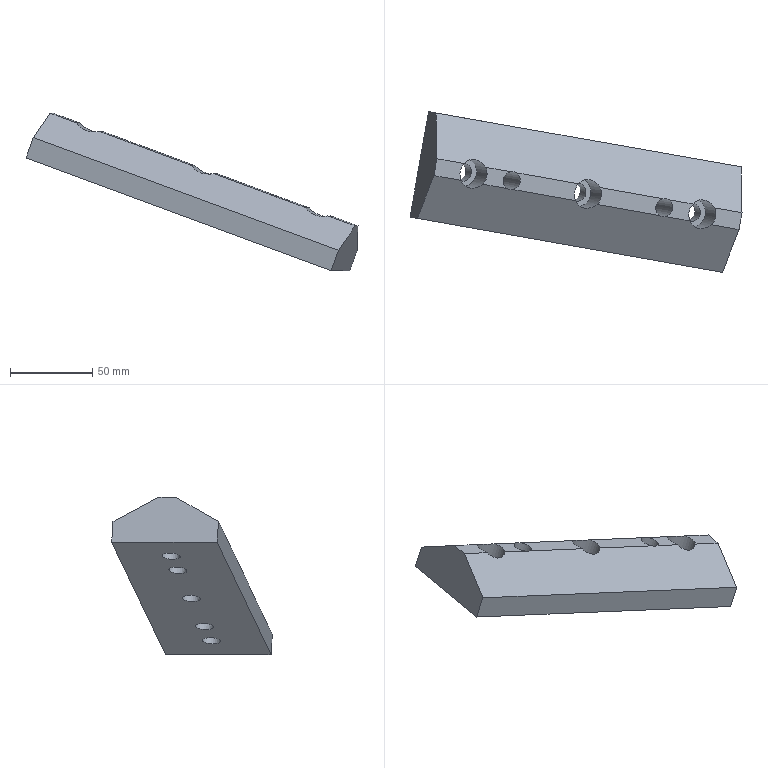Part | NX | features solid 2 | 1 solid | 24 faces | box 201.397 x 97.434 x 95.655 mm | volume 269020 mm3 | plane 16 | cylinder 8 | commonest cylinder face diameters 11 x5 17.5 x3
STEP:
#1=CARTESIAN_POINT('',(-972.407,367.24,-198.041));
#2=VERTEX_POINT('',#1);
#3=CARTESIAN_POINT('',(-1010.495,373.956,-183.964));
#4=VERTEX_POINT('',#3);
#5=CARTESIAN_POINT('',(-873.35,349.774,-234.651));
#6=DIRECTION('',(-0.9254,0.1632,0.342));
#7=VECTOR('',#6,1000.);
#8=LINE('',#5,#7);
#9=EDGE_CURVE('',#2,#4,#8,.T.);
#10=ORIENTED_EDGE('',*,*,#9,.T.);
#11=CARTESIAN_POINT('',(-1012.299,363.722,-183.964));
#12=VERTEX_POINT('',#11);
#13=CARTESIAN_POINT('',(-1013.065,369.133,-183.348));
#14=DIRECTION('',(-0.3368,0.05939,-0.9397));
#15=DIRECTION('',(-0.9254,0.1632,0.342));
#16=AXIS2_PLACEMENT_3D('',#13,#14,#15);
#17=CIRCLE('',#16,5.5);
#18=EDGE_CURVE('',#4,#12,#17,.T.);
#19=ORIENTED_EDGE('',*,*,#18,.T.);
#20=CARTESIAN_POINT('',(-974.212,357.006,-198.041));
#21=VERTEX_POINT('',#20);
#22=CARTESIAN_POINT('',(-875.155,339.54,-234.651));
#23=DIRECTION('',(-0.9254,0.1632,0.342));
#24=VECTOR('',#23,1000.);
#25=LINE('',#22,#24);
#26=EDGE_CURVE('',#21,#12,#25,.T.);
#27=ORIENTED_EDGE('',*,*,#26,.F.);
#28=CARTESIAN_POINT('',(-966.794,360.974,-200.449));
#29=DIRECTION('',(0.3368,-0.05939,0.9397));
#30=DIRECTION('',(0.9254,-0.1632,-0.342));
#31=AXIS2_PLACEMENT_3D('',#28,#29,#30);
#32=CIRCLE('',#31,8.75);
#33=EDGE_CURVE('',#2,#21,#32,.T.);
#34=ORIENTED_EDGE('',*,*,#33,.F.);
#35=EDGE_LOOP('',(#10,#19,#27,#34));
#36=FACE_BOUND('',#35,.T.);
#37=CARTESIAN_POINT('',(-875.155,339.54,-234.651));
#38=DIRECTION('',(0.3368,-0.05939,0.9397));
#39=DIRECTION('',(0.9254,-0.1632,-0.342));
#40=AXIS2_PLACEMENT_3D('',#37,#38,#39);
#41=PLANE('',#40);
#42=ADVANCED_FACE('',(#36),#41,.T.);
#43=CARTESIAN_POINT('',(-1051.058,375.832,-200.167));
#44=VERTEX_POINT('',#43);
#45=CARTESIAN_POINT('',(-1045.969,374.935,-202.048));
#46=DIRECTION('',(0.3368,-0.05939,0.9397));
#47=DIRECTION('',(-0.9254,0.1632,0.342));
#48=AXIS2_PLACEMENT_3D('',#45,#46,#47);
#49=CIRCLE('',#48,5.5);
#50=EDGE_CURVE('',#44,#44,#49,.T.);
#51=ORIENTED_EDGE('',*,*,#50,.T.);
#52=EDGE_LOOP('',(#51));
#53=FACE_BOUND('',#52,.T.);
#54=CARTESIAN_POINT('',(-1027.923,371.753,-208.718));
#55=VERTEX_POINT('',#54);
#56=CARTESIAN_POINT('',(-1022.833,370.855,-210.599));
#57=DIRECTION('',(-0.3368,0.05939,-0.9397));
#58=DIRECTION('',(-0.9254,0.1632,0.342));
#59=AXIS2_PLACEMENT_3D('',#56,#57,#58);
#60=CIRCLE('',#59,5.5);
#61=EDGE_CURVE('',#55,#55,#60,.T.);
#62=ORIENTED_EDGE('',*,*,#61,.F.);
#63=EDGE_LOOP('',(#62));
#64=FACE_BOUND('',#63,.T.);
#65=CARTESIAN_POINT('',(-981.652,363.594,-225.819));
#66=VERTEX_POINT('',#65);
#67=CARTESIAN_POINT('',(-976.562,362.697,-227.7));
#68=DIRECTION('',(0.3368,-0.05939,0.9397));
#69=DIRECTION('',(-0.9254,0.1632,0.342));
#70=AXIS2_PLACEMENT_3D('',#67,#68,#69);
#71=CIRCLE('',#70,5.5);
#72=EDGE_CURVE('',#66,#66,#71,.T.);
#73=ORIENTED_EDGE('',*,*,#72,.T.);
#74=EDGE_LOOP('',(#73));
#75=FACE_BOUND('',#74,.T.);
#76=CARTESIAN_POINT('',(-889.664,314.373,-261.902));
#77=VERTEX_POINT('',#76);
#78=CARTESIAN_POINT('',(-1074.747,347.008,-193.498));
#79=VERTEX_POINT('',#78);
#80=CARTESIAN_POINT('',(-889.664,314.373,-261.902));
#81=DIRECTION('',(-0.9254,0.1632,0.342));
#82=VECTOR('',#81,1000.);
#83=LINE('',#80,#82);
#84=EDGE_CURVE('',#77,#79,#83,.T.);
#85=ORIENTED_EDGE('',*,*,#84,.T.);
#86=CARTESIAN_POINT('',(-1063.46,411.021,-193.498));
#87=VERTEX_POINT('',#86);
#88=CARTESIAN_POINT('',(-1074.747,347.008,-193.498));
#89=DIRECTION('',(0.1736,0.9848,0.));
#90=VECTOR('',#89,1000.);
#91=LINE('',#88,#90);
#92=EDGE_CURVE('',#79,#87,#91,.T.);
#93=ORIENTED_EDGE('',*,*,#92,.T.);
#94=CARTESIAN_POINT('',(-878.377,378.385,-261.902));
#95=VERTEX_POINT('',#94);
#96=CARTESIAN_POINT('',(-878.377,378.385,-261.902));
#97=DIRECTION('',(-0.9254,0.1632,0.342));
#98=VECTOR('',#97,1000.);
#99=LINE('',#96,#98);
#100=EDGE_CURVE('',#95,#87,#99,.T.);
#101=ORIENTED_EDGE('',*,*,#100,.F.);
#102=CARTESIAN_POINT('',(-889.664,314.373,-261.902));
#103=DIRECTION('',(0.1736,0.9848,0.));
#104=VECTOR('',#103,1000.);
#105=LINE('',#102,#104);
#106=EDGE_CURVE('',#77,#95,#105,.T.);
#107=ORIENTED_EDGE('',*,*,#106,.F.);
#108=EDGE_LOOP('',(#85,#93,#101,#107));
#109=FACE_BOUND('',#108,.T.);
#110=CARTESIAN_POINT('',(-935.381,355.435,-242.92));
#111=VERTEX_POINT('',#110);
#112=CARTESIAN_POINT('',(-930.291,354.538,-244.801));
#113=DIRECTION('',(-0.3368,0.05939,-0.9397));
#114=DIRECTION('',(-0.9254,0.1632,0.342));
#115=AXIS2_PLACEMENT_3D('',#112,#113,#114);
#116=CIRCLE('',#115,5.5);
#117=EDGE_CURVE('',#111,#111,#116,.T.);
#118=ORIENTED_EDGE('',*,*,#117,.F.);
#119=EDGE_LOOP('',(#118));
#120=FACE_BOUND('',#119,.T.);
#121=CARTESIAN_POINT('',(-912.246,351.356,-251.47));
#122=VERTEX_POINT('',#121);
#123=CARTESIAN_POINT('',(-907.156,350.459,-253.351));
#124=DIRECTION('',(0.3368,-0.05939,0.9397));
#125=DIRECTION('',(-0.9254,0.1632,0.342));
#126=AXIS2_PLACEMENT_3D('',#123,#124,#125);
#127=CIRCLE('',#126,5.5);
#128=EDGE_CURVE('',#122,#122,#127,.T.);
#129=ORIENTED_EDGE('',*,*,#128,.T.);
#130=EDGE_LOOP('',(#129));
#131=FACE_BOUND('',#130,.T.);
#132=CARTESIAN_POINT('',(-889.664,314.373,-261.902));
#133=DIRECTION('',(0.3368,-0.05939,0.9397));
#134=DIRECTION('',(-0.1736,-0.9848,0.));
#135=AXIS2_PLACEMENT_3D('',#132,#133,#134);
#136=PLANE('',#135);
#137=ADVANCED_FACE('',(#53,#64,#75,#109,#120,#131),#136,.F.);
#138=CARTESIAN_POINT('',(-1013.831,374.545,-182.731));
#139=VERTEX_POINT('',#138);
#140=CARTESIAN_POINT('',(-1012.055,368.955,-180.529));
#141=DIRECTION('',(0.3785,0.441,0.8138));
#142=DIRECTION('',(-0.01803,0.8826,-0.4698));
#143=AXIS2_PLACEMENT_3D('',#140,#141,#142);
#144=ELLIPSE('',#143,6.351,5.5);
#145=EDGE_CURVE('',#4,#139,#144,.T.);
#146=ORIENTED_EDGE('',*,*,#145,.F.);
#147=ORIENTED_EDGE('',*,*,#9,.F.);
#148=CARTESIAN_POINT('',(-959.377,364.943,-202.857));
#149=VERTEX_POINT('',#148);
#150=CARTESIAN_POINT('',(-965.784,360.796,-197.63));
#151=DIRECTION('',(0.3785,0.441,0.8138));
#152=DIRECTION('',(-0.01803,0.8826,-0.4698));
#153=AXIS2_PLACEMENT_3D('',#150,#151,#152);
#154=ELLIPSE('',#153,10.104,8.75);
#155=EDGE_CURVE('',#149,#2,#154,.T.);
#156=ORIENTED_EDGE('',*,*,#155,.F.);
#157=CARTESIAN_POINT('',(-921.29,358.227,-216.933));
#158=VERTEX_POINT('',#157);
#159=CARTESIAN_POINT('',(-873.35,349.774,-234.651));
#160=DIRECTION('',(-0.9254,0.1632,0.342));
#161=VECTOR('',#160,1000.);
#162=LINE('',#159,#161);
#163=EDGE_CURVE('',#158,#149,#162,.T.);
#164=ORIENTED_EDGE('',*,*,#163,.F.);
#165=CARTESIAN_POINT('',(-917.953,357.639,-218.166));
#166=VERTEX_POINT('',#165);
#167=CARTESIAN_POINT('',(-919.513,352.637,-214.731));
#168=DIRECTION('',(0.3785,0.441,0.8138));
#169=DIRECTION('',(-0.01803,0.8826,-0.4698));
#170=AXIS2_PLACEMENT_3D('',#167,#168,#169);
#171=ELLIPSE('',#170,6.351,5.5);
#172=EDGE_CURVE('',#166,#158,#171,.T.);
#173=ORIENTED_EDGE('',*,*,#172,.F.);
#174=CARTESIAN_POINT('',(-903.001,355.002,-223.692));
#175=VERTEX_POINT('',#174);
#176=CARTESIAN_POINT('',(-873.35,349.774,-234.651));
#177=DIRECTION('',(-0.9254,0.1632,0.342));
#178=VECTOR('',#177,1000.);
#179=LINE('',#176,#178);
#180=EDGE_CURVE('',#175,#166,#179,.T.);
#181=ORIENTED_EDGE('',*,*,#180,.F.);
#182=CARTESIAN_POINT('',(-889.971,352.705,-228.508));
#183=VERTEX_POINT('',#182);
#184=CARTESIAN_POINT('',(-896.378,348.558,-223.281));
#185=DIRECTION('',(0.3785,0.441,0.8138));
#186=DIRECTION('',(-0.01803,0.8826,-0.4698));
#187=AXIS2_PLACEMENT_3D('',#184,#185,#186);
#188=ELLIPSE('',#187,10.104,8.75);
#189=EDGE_CURVE('',#183,#175,#188,.T.);
#190=ORIENTED_EDGE('',*,*,#189,.F.);
#191=CARTESIAN_POINT('',(-873.35,349.774,-234.651));
#192=VERTEX_POINT('',#191);
#193=CARTESIAN_POINT('',(-873.35,349.774,-234.651));
#194=DIRECTION('',(-0.9254,0.1632,0.342));
#195=VECTOR('',#194,1000.);
#196=LINE('',#193,#195);
#197=EDGE_CURVE('',#192,#183,#196,.T.);
#198=ORIENTED_EDGE('',*,*,#197,.F.);
#199=CARTESIAN_POINT('',(-873.919,377.599,-249.464));
#200=VERTEX_POINT('',#199);
#201=CARTESIAN_POINT('',(-873.35,349.774,-234.651));
#202=DIRECTION('',(-0.01803,0.8826,-0.4698));
#203=VECTOR('',#202,1000.);
#204=LINE('',#201,#203);
#205=EDGE_CURVE('',#192,#200,#204,.T.);
#206=ORIENTED_EDGE('',*,*,#205,.T.);
#207=CARTESIAN_POINT('',(-1059.002,410.234,-181.06));
#208=VERTEX_POINT('',#207);
#209=CARTESIAN_POINT('',(-873.919,377.599,-249.464));
#210=DIRECTION('',(-0.9254,0.1632,0.342));
#211=VECTOR('',#210,1000.);
#212=LINE('',#209,#211);
#213=EDGE_CURVE('',#200,#208,#212,.T.);
#214=ORIENTED_EDGE('',*,*,#213,.T.);
#215=CARTESIAN_POINT('',(-1058.434,382.409,-166.247));
#216=VERTEX_POINT('',#215);
#217=CARTESIAN_POINT('',(-1058.434,382.409,-166.247));
#218=DIRECTION('',(-0.01803,0.8826,-0.4698));
#219=VECTOR('',#218,1000.);
#220=LINE('',#217,#219);
#221=EDGE_CURVE('',#216,#208,#220,.T.);
#222=ORIENTED_EDGE('',*,*,#221,.F.);
#223=CARTESIAN_POINT('',(-1041.813,379.479,-172.389));
#224=VERTEX_POINT('',#223);
#225=CARTESIAN_POINT('',(-873.35,349.774,-234.651));
#226=DIRECTION('',(-0.9254,0.1632,0.342));
#227=VECTOR('',#226,1000.);
#228=LINE('',#225,#227);
#229=EDGE_CURVE('',#224,#216,#228,.T.);
#230=ORIENTED_EDGE('',*,*,#229,.F.);
#231=CARTESIAN_POINT('',(-1028.783,377.181,-177.205));
#232=VERTEX_POINT('',#231);
#233=CARTESIAN_POINT('',(-1035.19,373.034,-171.978));
#234=DIRECTION('',(0.3785,0.441,0.8138));
#235=DIRECTION('',(-0.01803,0.8826,-0.4698));
#236=AXIS2_PLACEMENT_3D('',#233,#234,#235);
#237=ELLIPSE('',#236,10.104,8.75);
#238=EDGE_CURVE('',#232,#224,#237,.T.);
#239=ORIENTED_EDGE('',*,*,#238,.F.);
#240=CARTESIAN_POINT('',(-873.35,349.774,-234.651));
#241=DIRECTION('',(-0.9254,0.1632,0.342));
#242=VECTOR('',#241,1000.);
#243=LINE('',#240,#242);
#244=EDGE_CURVE('',#139,#232,#243,.T.);
#245=ORIENTED_EDGE('',*,*,#244,.F.);
#246=EDGE_LOOP('',(#146,#147,#156,#164,#173,#181,#190,#198,#206,#214,#222,#230,#239,#245));
#247=FACE_BOUND('',#246,.T.);
#248=CARTESIAN_POINT('',(-873.35,349.774,-234.651));
#249=DIRECTION('',(0.3785,0.441,0.8138));
#250=DIRECTION('',(0.01803,-0.8826,0.4698));
#251=AXIS2_PLACEMENT_3D('',#248,#249,#250);
#252=PLANE('',#251);
#253=ADVANCED_FACE('',(#247),#252,.T.);
#254=ORIENTED_EDGE('',*,*,#26,.T.);
#255=CARTESIAN_POINT('',(-1015.636,364.31,-182.731));
#256=VERTEX_POINT('',#255);
#257=CARTESIAN_POINT('',(-1012.055,368.955,-180.529));
#258=DIRECTION('',(-0.2049,0.5438,-0.8138));
#259=DIRECTION('',(-0.3188,-0.8232,-0.4698));
#260=AXIS2_PLACEMENT_3D('',#257,#258,#259);
#261=ELLIPSE('',#260,6.351,5.5);
#262=EDGE_CURVE('',#12,#256,#261,.T.);
#263=ORIENTED_EDGE('',*,*,#262,.T.);
#264=CARTESIAN_POINT('',(-1030.588,366.947,-177.205));
#265=VERTEX_POINT('',#264);
#266=CARTESIAN_POINT('',(-875.155,339.54,-234.651));
#267=DIRECTION('',(-0.9254,0.1632,0.342));
#268=VECTOR('',#267,1000.);
#269=LINE('',#266,#268);
#270=EDGE_CURVE('',#256,#265,#269,.T.);
#271=ORIENTED_EDGE('',*,*,#270,.T.);
#272=CARTESIAN_POINT('',(-1043.618,369.244,-172.389));
#273=VERTEX_POINT('',#272);
#274=CARTESIAN_POINT('',(-1035.19,373.034,-171.978));
#275=DIRECTION('',(-0.2049,0.5438,-0.8138));
#276=DIRECTION('',(-0.3188,-0.8232,-0.4698));
#277=AXIS2_PLACEMENT_3D('',#274,#275,#276);
#278=ELLIPSE('',#277,10.104,8.75);
#279=EDGE_CURVE('',#265,#273,#278,.T.);
#280=ORIENTED_EDGE('',*,*,#279,.T.);
#281=CARTESIAN_POINT('',(-1060.238,372.175,-166.247));
#282=VERTEX_POINT('',#281);
#283=CARTESIAN_POINT('',(-875.155,339.54,-234.651));
#284=DIRECTION('',(-0.9254,0.1632,0.342));
#285=VECTOR('',#284,1000.);
#286=LINE('',#283,#285);
#287=EDGE_CURVE('',#273,#282,#286,.T.);
#288=ORIENTED_EDGE('',*,*,#287,.T.);
#289=CARTESIAN_POINT('',(-1070.289,346.222,-181.06));
#290=VERTEX_POINT('',#289);
#291=CARTESIAN_POINT('',(-1060.238,372.175,-166.247));
#292=DIRECTION('',(-0.3188,-0.8232,-0.4698));
#293=VECTOR('',#292,1000.);
#294=LINE('',#291,#293);
#295=EDGE_CURVE('',#282,#290,#294,.T.);
#296=ORIENTED_EDGE('',*,*,#295,.T.);
#297=CARTESIAN_POINT('',(-885.206,313.587,-249.464));
#298=VERTEX_POINT('',#297);
#299=CARTESIAN_POINT('',(-885.206,313.587,-249.464));
#300=DIRECTION('',(-0.9254,0.1632,0.342));
#301=VECTOR('',#300,1000.);
#302=LINE('',#299,#301);
#303=EDGE_CURVE('',#298,#290,#302,.T.);
#304=ORIENTED_EDGE('',*,*,#303,.F.);
#305=CARTESIAN_POINT('',(-875.155,339.54,-234.651));
#306=VERTEX_POINT('',#305);
#307=CARTESIAN_POINT('',(-875.155,339.54,-234.651));
#308=DIRECTION('',(-0.3188,-0.8232,-0.4698));
#309=VECTOR('',#308,1000.);
#310=LINE('',#307,#309);
#311=EDGE_CURVE('',#306,#298,#310,.T.);
#312=ORIENTED_EDGE('',*,*,#311,.F.);
#313=CARTESIAN_POINT('',(-891.775,342.47,-228.508));
#314=VERTEX_POINT('',#313);
#315=CARTESIAN_POINT('',(-875.155,339.54,-234.651));
#316=DIRECTION('',(-0.9254,0.1632,0.342));
#317=VECTOR('',#316,1000.);
#318=LINE('',#315,#317);
#319=EDGE_CURVE('',#306,#314,#318,.T.);
#320=ORIENTED_EDGE('',*,*,#319,.T.);
#321=CARTESIAN_POINT('',(-904.805,344.768,-223.692));
#322=VERTEX_POINT('',#321);
#323=CARTESIAN_POINT('',(-896.378,348.558,-223.281));
#324=DIRECTION('',(-0.2049,0.5438,-0.8138));
#325=DIRECTION('',(-0.3188,-0.8232,-0.4698));
#326=AXIS2_PLACEMENT_3D('',#323,#324,#325);
#327=ELLIPSE('',#326,10.104,8.75);
#328=EDGE_CURVE('',#314,#322,#327,.T.);
#329=ORIENTED_EDGE('',*,*,#328,.T.);
#330=CARTESIAN_POINT('',(-919.758,347.404,-218.166));
#331=VERTEX_POINT('',#330);
#332=CARTESIAN_POINT('',(-875.155,339.54,-234.651));
#333=DIRECTION('',(-0.9254,0.1632,0.342));
#334=VECTOR('',#333,1000.);
#335=LINE('',#332,#334);
#336=EDGE_CURVE('',#322,#331,#335,.T.);
#337=ORIENTED_EDGE('',*,*,#336,.T.);
#338=CARTESIAN_POINT('',(-923.094,347.993,-216.933));
#339=VERTEX_POINT('',#338);
#340=CARTESIAN_POINT('',(-919.513,352.637,-214.731));
#341=DIRECTION('',(-0.2049,0.5438,-0.8138));
#342=DIRECTION('',(-0.3188,-0.8232,-0.4698));
#343=AXIS2_PLACEMENT_3D('',#340,#341,#342);
#344=ELLIPSE('',#343,6.351,5.5);
#345=EDGE_CURVE('',#331,#339,#344,.T.);
#346=ORIENTED_EDGE('',*,*,#345,.T.);
#347=CARTESIAN_POINT('',(-961.182,354.708,-202.857));
#348=VERTEX_POINT('',#347);
#349=CARTESIAN_POINT('',(-875.155,339.54,-234.651));
#350=DIRECTION('',(-0.9254,0.1632,0.342));
#351=VECTOR('',#350,1000.);
#352=LINE('',#349,#351);
#353=EDGE_CURVE('',#339,#348,#352,.T.);
#354=ORIENTED_EDGE('',*,*,#353,.T.);
#355=CARTESIAN_POINT('',(-965.784,360.796,-197.63));
#356=DIRECTION('',(-0.2049,0.5438,-0.8138));
#357=DIRECTION('',(-0.3188,-0.8232,-0.4698));
#358=AXIS2_PLACEMENT_3D('',#355,#356,#357);
#359=ELLIPSE('',#358,10.104,8.75);
#360=EDGE_CURVE('',#348,#21,#359,.T.);
#361=ORIENTED_EDGE('',*,*,#360,.T.);
#362=EDGE_LOOP('',(#254,#263,#271,#280,#288,#296,#304,#312,#320,#329,#337,#346,#354,#361));
#363=FACE_BOUND('',#362,.T.);
#364=CARTESIAN_POINT('',(-875.155,339.54,-234.651));
#365=DIRECTION('',(0.2049,-0.5438,0.8138));
#366=DIRECTION('',(0.3188,0.8232,0.4698));
#367=AXIS2_PLACEMENT_3D('',#364,#365,#366);
#368=PLANE('',#367);
#369=ADVANCED_FACE('',(#363),#368,.T.);
#370=CARTESIAN_POINT('',(-966.794,360.974,-200.449));
#371=DIRECTION('',(-0.3368,0.05939,-0.9397));
#372=DIRECTION('',(-0.9254,0.1632,0.342));
#373=AXIS2_PLACEMENT_3D('',#370,#371,#372);
#374=CIRCLE('',#373,8.75);
#375=EDGE_CURVE('',#149,#348,#374,.T.);
#376=ORIENTED_EDGE('',*,*,#375,.T.);
#377=ORIENTED_EDGE('',*,*,#353,.F.);
#378=CARTESIAN_POINT('',(-920.524,352.816,-217.55));
#379=DIRECTION('',(-0.3368,0.05939,-0.9397));
#380=DIRECTION('',(-0.9254,0.1632,0.342));
#381=AXIS2_PLACEMENT_3D('',#378,#379,#380);
#382=CIRCLE('',#381,5.5);
#383=EDGE_CURVE('',#339,#158,#382,.T.);
#384=ORIENTED_EDGE('',*,*,#383,.T.);
#385=ORIENTED_EDGE('',*,*,#163,.T.);
#386=EDGE_LOOP('',(#376,#377,#384,#385));
#387=FACE_BOUND('',#386,.T.);
#388=CARTESIAN_POINT('',(-875.155,339.54,-234.651));
#389=DIRECTION('',(0.3368,-0.05939,0.9397));
#390=DIRECTION('',(0.9254,-0.1632,-0.342));
#391=AXIS2_PLACEMENT_3D('',#388,#389,#390);
#392=PLANE('',#391);
#393=ADVANCED_FACE('',(#387),#392,.T.);
#394=CARTESIAN_POINT('',(-920.524,352.816,-217.55));
#395=DIRECTION('',(-0.3368,0.05939,-0.9397));
#396=DIRECTION('',(-0.9254,0.1632,0.342));
#397=AXIS2_PLACEMENT_3D('',#394,#395,#396);
#398=CIRCLE('',#397,5.5);
#399=EDGE_CURVE('',#166,#331,#398,.T.);
#400=ORIENTED_EDGE('',*,*,#399,.T.);
#401=ORIENTED_EDGE('',*,*,#336,.F.);
#402=CARTESIAN_POINT('',(-897.388,348.736,-226.1));
#403=DIRECTION('',(0.3368,-0.05939,0.9397));
#404=DIRECTION('',(0.9254,-0.1632,-0.342));
#405=AXIS2_PLACEMENT_3D('',#402,#403,#404);
#406=CIRCLE('',#405,8.75);
#407=EDGE_CURVE('',#175,#322,#406,.T.);
#408=ORIENTED_EDGE('',*,*,#407,.F.);
#409=ORIENTED_EDGE('',*,*,#180,.T.);
#410=EDGE_LOOP('',(#400,#401,#408,#409));
#411=FACE_BOUND('',#410,.T.);
#412=CARTESIAN_POINT('',(-875.155,339.54,-234.651));
#413=DIRECTION('',(0.3368,-0.05939,0.9397));
#414=DIRECTION('',(0.9254,-0.1632,-0.342));
#415=AXIS2_PLACEMENT_3D('',#412,#413,#414);
#416=PLANE('',#415);
#417=ADVANCED_FACE('',(#411),#416,.T.);
#418=CARTESIAN_POINT('',(-1036.201,373.213,-174.797));
#419=DIRECTION('',(-0.3368,0.05939,-0.9397));
#420=DIRECTION('',(-0.9254,0.1632,0.342));
#421=AXIS2_PLACEMENT_3D('',#418,#419,#420);
#422=CIRCLE('',#421,8.75);
#423=EDGE_CURVE('',#232,#265,#422,.T.);
#424=ORIENTED_EDGE('',*,*,#423,.T.);
#425=ORIENTED_EDGE('',*,*,#270,.F.);
#426=CARTESIAN_POINT('',(-1013.065,369.133,-183.348));
#427=DIRECTION('',(0.3368,-0.05939,0.9397));
#428=DIRECTION('',(0.9254,-0.1632,-0.342));
#429=AXIS2_PLACEMENT_3D('',#426,#427,#428);
#430=CIRCLE('',#429,5.5);
#431=EDGE_CURVE('',#139,#256,#430,.T.);
#432=ORIENTED_EDGE('',*,*,#431,.F.);
#433=ORIENTED_EDGE('',*,*,#244,.T.);
#434=EDGE_LOOP('',(#424,#425,#432,#433));
#435=FACE_BOUND('',#434,.T.);
#436=CARTESIAN_POINT('',(-875.155,339.54,-234.651));
#437=DIRECTION('',(0.3368,-0.05939,0.9397));
#438=DIRECTION('',(0.9254,-0.1632,-0.342));
#439=AXIS2_PLACEMENT_3D('',#436,#437,#438);
#440=PLANE('',#439);
#441=ADVANCED_FACE('',(#435),#440,.T.);
#442=CARTESIAN_POINT('',(-1060.238,372.175,-166.247));
#443=DIRECTION('',(0.1736,0.9848,0.));
#444=VECTOR('',#443,1000.);
#445=LINE('',#442,#444);
#446=EDGE_CURVE('',#282,#216,#445,.T.);
#447=ORIENTED_EDGE('',*,*,#446,.F.);
#448=ORIENTED_EDGE('',*,*,#287,.F.);
#449=CARTESIAN_POINT('',(-1036.201,373.213,-174.797));
#450=DIRECTION('',(0.3368,-0.05939,0.9397));
#451=DIRECTION('',(0.9254,-0.1632,-0.342));
#452=AXIS2_PLACEMENT_3D('',#449,#450,#451);
#453=CIRCLE('',#452,8.75);
#454=EDGE_CURVE('',#224,#273,#453,.T.);
#455=ORIENTED_EDGE('',*,*,#454,.F.);
#456=ORIENTED_EDGE('',*,*,#229,.T.);
#457=EDGE_LOOP('',(#447,#448,#455,#456));
#458=FACE_BOUND('',#457,.T.);
#459=CARTESIAN_POINT('',(-875.155,339.54,-234.651));
#460=DIRECTION('',(0.3368,-0.05939,0.9397));
#461=DIRECTION('',(0.9254,-0.1632,-0.342));
#462=AXIS2_PLACEMENT_3D('',#459,#460,#461);
#463=PLANE('',#462);
#464=ADVANCED_FACE('',(#458),#463,.T.);
#465=CARTESIAN_POINT('',(-897.388,348.736,-226.1));
#466=DIRECTION('',(-0.3368,0.05939,-0.9397));
#467=DIRECTION('',(-0.9254,0.1632,0.342));
#468=AXIS2_PLACEMENT_3D('',#465,#466,#467);
#469=CIRCLE('',#468,8.75);
#470=EDGE_CURVE('',#183,#314,#469,.T.);
#471=ORIENTED_EDGE('',*,*,#470,.T.);
#472=ORIENTED_EDGE('',*,*,#319,.F.);
#473=CARTESIAN_POINT('',(-875.155,339.54,-234.651));
#474=DIRECTION('',(0.1736,0.9848,0.));
#475=VECTOR('',#474,1000.);
#476=LINE('',#473,#475);
#477=EDGE_CURVE('',#306,#192,#476,.T.);
#478=ORIENTED_EDGE('',*,*,#477,.T.);
#479=ORIENTED_EDGE('',*,*,#197,.T.);
#480=EDGE_LOOP('',(#471,#472,#478,#479));
#481=FACE_BOUND('',#480,.T.);
#482=CARTESIAN_POINT('',(-875.155,339.54,-234.651));
#483=DIRECTION('',(0.3368,-0.05939,0.9397));
#484=DIRECTION('',(0.9254,-0.1632,-0.342));
#485=AXIS2_PLACEMENT_3D('',#482,#483,#484);
#486=PLANE('',#485);
#487=ADVANCED_FACE('',(#481),#486,.T.);
#488=ORIENTED_EDGE('',*,*,#477,.F.);
#489=ORIENTED_EDGE('',*,*,#311,.T.);
#490=CARTESIAN_POINT('',(-894.717,315.264,-275.997));
#491=DIRECTION('',(0.3368,-0.05939,0.9397));
#492=VECTOR('',#491,1000.);
#493=LINE('',#490,#492);
#494=EDGE_CURVE('',#77,#298,#493,.T.);
#495=ORIENTED_EDGE('',*,*,#494,.F.);
#496=ORIENTED_EDGE('',*,*,#106,.T.);
#497=CARTESIAN_POINT('',(-883.429,379.276,-275.997));
#498=DIRECTION('',(0.3368,-0.05939,0.9397));
#499=VECTOR('',#498,1000.);
#500=LINE('',#497,#499);
#501=EDGE_CURVE('',#95,#200,#500,.T.);
#502=ORIENTED_EDGE('',*,*,#501,.T.);
#503=ORIENTED_EDGE('',*,*,#205,.F.);
#504=EDGE_LOOP('',(#488,#489,#495,#496,#502,#503));
#505=FACE_BOUND('',#504,.T.);
#506=CARTESIAN_POINT('',(-873.242,344.479,-231.832));
#507=DIRECTION('',(0.9254,-0.1632,-0.342));
#508=DIRECTION('',(-0.3368,0.05939,-0.9397));
#509=AXIS2_PLACEMENT_3D('',#506,#507,#508);
#510=PLANE('',#509);
#511=ADVANCED_FACE('',(#505),#510,.T.);
#512=ORIENTED_EDGE('',*,*,#446,.T.);
#513=ORIENTED_EDGE('',*,*,#221,.T.);
#514=CARTESIAN_POINT('',(-1068.513,411.911,-207.593));
#515=DIRECTION('',(0.3368,-0.05939,0.9397));
#516=VECTOR('',#515,1000.);
#517=LINE('',#514,#516);
#518=EDGE_CURVE('',#87,#208,#517,.T.);
#519=ORIENTED_EDGE('',*,*,#518,.F.);
#520=ORIENTED_EDGE('',*,*,#92,.F.);
#521=CARTESIAN_POINT('',(-1079.8,347.899,-207.593));
#522=DIRECTION('',(0.3368,-0.05939,0.9397));
#523=VECTOR('',#522,1000.);
#524=LINE('',#521,#523);
#525=EDGE_CURVE('',#79,#290,#524,.T.);
#526=ORIENTED_EDGE('',*,*,#525,.T.);
#527=ORIENTED_EDGE('',*,*,#295,.F.);
#528=EDGE_LOOP('',(#512,#513,#519,#520,#526,#527));
#529=FACE_BOUND('',#528,.T.);
#530=CARTESIAN_POINT('',(-1058.326,377.114,-163.428));
#531=DIRECTION('',(0.9254,-0.1632,-0.342));
#532=DIRECTION('',(-0.3368,0.05939,-0.9397));
#533=AXIS2_PLACEMENT_3D('',#530,#531,#532);
#534=PLANE('',#533);
#535=ADVANCED_FACE('',(#529),#534,.F.);
#536=ORIENTED_EDGE('',*,*,#50,.F.);
#537=EDGE_LOOP('',(#536));
#538=FACE_BOUND('',#537,.T.);
#539=CARTESIAN_POINT('',(-1047.778,374.341,-190.796));
#540=VERTEX_POINT('',#539);
#541=CARTESIAN_POINT('',(-1042.6,374.341,-192.651));
#542=DIRECTION('',(-0.3368,0.05939,-0.9397));
#543=DIRECTION('',(-0.9414,0.,0.3374));
#544=AXIS2_PLACEMENT_3D('',#541,#542,#543);
#545=CIRCLE('',#544,5.5);
#546=EDGE_CURVE('',#540,#540,#545,.T.);
#547=ORIENTED_EDGE('',*,*,#546,.F.);
#548=EDGE_LOOP('',(#547));
#549=FACE_BOUND('',#548,.T.);
#550=CARTESIAN_POINT('',(-1052.031,376.004,-218.963));
#551=DIRECTION('',(-0.3368,0.05939,-0.9397));
#552=DIRECTION('',(-0.9254,0.1632,0.342));
#553=AXIS2_PLACEMENT_3D('',#550,#551,#552);
#554=CYLINDRICAL_SURFACE('',#553,5.5);
#555=ADVANCED_FACE('',(#538,#549),#554,.F.);
#556=ORIENTED_EDGE('',*,*,#546,.T.);
#557=EDGE_LOOP('',(#556));
#558=FACE_BOUND('',#557,.T.);
#559=CARTESIAN_POINT('',(-1050.837,374.341,-189.699));
#560=VERTEX_POINT('',#559);
#561=CARTESIAN_POINT('',(-1042.6,374.341,-192.651));
#562=DIRECTION('',(-0.3368,0.05939,-0.9397));
#563=DIRECTION('',(-0.9414,0.,0.3374));
#564=AXIS2_PLACEMENT_3D('',#561,#562,#563);
#565=CIRCLE('',#564,8.75);
#566=EDGE_CURVE('',#560,#560,#565,.T.);
#567=ORIENTED_EDGE('',*,*,#566,.F.);
#568=EDGE_LOOP('',(#567));
#569=FACE_BOUND('',#568,.T.);
#570=CARTESIAN_POINT('',(-996.329,366.182,-209.752));
#571=DIRECTION('',(-0.3368,0.05939,-0.9397));
#572=DIRECTION('',(-0.9254,0.1632,0.342));
#573=AXIS2_PLACEMENT_3D('',#570,#571,#572);
#574=PLANE('',#573);
#575=ADVANCED_FACE('',(#558,#569),#574,.F.);
#576=ORIENTED_EDGE('',*,*,#566,.T.);
#577=EDGE_LOOP('',(#576));
#578=FACE_BOUND('',#577,.T.);
#579=ORIENTED_EDGE('',*,*,#423,.F.);
#580=ORIENTED_EDGE('',*,*,#238,.T.);
#581=ORIENTED_EDGE('',*,*,#454,.T.);
#582=ORIENTED_EDGE('',*,*,#279,.F.);
#583=EDGE_LOOP('',(#579,#580,#581,#582));
#584=FACE_BOUND('',#583,.T.);
#585=CARTESIAN_POINT('',(-1036.201,373.213,-174.797));
#586=DIRECTION('',(-0.3368,0.05939,-0.9397));
#587=DIRECTION('',(-0.9254,0.1632,0.342));
#588=AXIS2_PLACEMENT_3D('',#585,#586,#587);
#589=CYLINDRICAL_SURFACE('',#588,8.75);
#590=ADVANCED_FACE('',(#578,#584),#589,.F.);
#591=ORIENTED_EDGE('',*,*,#61,.T.);
#592=EDGE_LOOP('',(#591));
#593=FACE_BOUND('',#592,.T.);
#594=ORIENTED_EDGE('',*,*,#18,.F.);
#595=ORIENTED_EDGE('',*,*,#145,.T.);
#596=ORIENTED_EDGE('',*,*,#431,.T.);
#597=ORIENTED_EDGE('',*,*,#262,.F.);
#598=EDGE_LOOP('',(#594,#595,#596,#597));
#599=FACE_BOUND('',#598,.T.);
#600=CARTESIAN_POINT('',(-1013.065,369.133,-183.348));
#601=DIRECTION('',(-0.3368,0.05939,-0.9397));
#602=DIRECTION('',(-0.9254,0.1632,0.342));
#603=AXIS2_PLACEMENT_3D('',#600,#601,#602);
#604=CYLINDRICAL_SURFACE('',#603,5.5);
#605=ADVANCED_FACE('',(#593,#599),#604,.F.);
#606=ORIENTED_EDGE('',*,*,#72,.F.);
#607=EDGE_LOOP('',(#606));
#608=FACE_BOUND('',#607,.T.);
#609=CARTESIAN_POINT('',(-978.371,362.103,-216.447));
#610=VERTEX_POINT('',#609);
#611=CARTESIAN_POINT('',(-973.194,362.103,-218.303));
#612=DIRECTION('',(-0.3368,0.05939,-0.9397));
#613=DIRECTION('',(-0.9414,0.,0.3374));
#614=AXIS2_PLACEMENT_3D('',#611,#612,#613);
#615=CIRCLE('',#614,5.5);
#616=EDGE_CURVE('',#610,#610,#615,.T.);
#617=ORIENTED_EDGE('',*,*,#616,.F.);
#618=EDGE_LOOP('',(#617));
#619=FACE_BOUND('',#618,.T.);
#620=CARTESIAN_POINT('',(-982.625,363.766,-244.614));
#621=DIRECTION('',(-0.3368,0.05939,-0.9397));
#622=DIRECTION('',(-0.9254,0.1632,0.342));
#623=AXIS2_PLACEMENT_3D('',#620,#621,#622);
#624=CYLINDRICAL_SURFACE('',#623,5.5);
#625=ADVANCED_FACE('',(#608,#619),#624,.F.);
#626=ORIENTED_EDGE('',*,*,#616,.T.);
#627=EDGE_LOOP('',(#626));
#628=FACE_BOUND('',#627,.T.);
#629=CARTESIAN_POINT('',(-981.431,362.103,-215.351));
#630=VERTEX_POINT('',#629);
#631=CARTESIAN_POINT('',(-973.194,362.103,-218.303));
#632=DIRECTION('',(-0.3368,0.05939,-0.9397));
#633=DIRECTION('',(-0.9414,0.,0.3374));
#634=AXIS2_PLACEMENT_3D('',#631,#632,#633);
#635=CIRCLE('',#634,8.75);
#636=EDGE_CURVE('',#630,#630,#635,.T.);
#637=ORIENTED_EDGE('',*,*,#636,.F.);
#638=EDGE_LOOP('',(#637));
#639=FACE_BOUND('',#638,.T.);
#640=CARTESIAN_POINT('',(-973.194,362.103,-218.303));
#641=DIRECTION('',(-0.3368,0.05939,-0.9397));
#642=DIRECTION('',(-0.9254,0.1632,0.342));
#643=AXIS2_PLACEMENT_3D('',#640,#641,#642);
#644=PLANE('',#643);
#645=ADVANCED_FACE('',(#628,#639),#644,.F.);
#646=ORIENTED_EDGE('',*,*,#636,.T.);
#647=EDGE_LOOP('',(#646));
#648=FACE_BOUND('',#647,.T.);
#649=ORIENTED_EDGE('',*,*,#375,.F.);
#650=ORIENTED_EDGE('',*,*,#155,.T.);
#651=ORIENTED_EDGE('',*,*,#33,.T.);
#652=ORIENTED_EDGE('',*,*,#360,.F.);
#653=EDGE_LOOP('',(#649,#650,#651,#652));
#654=FACE_BOUND('',#653,.T.);
#655=CARTESIAN_POINT('',(-966.794,360.974,-200.449));
#656=DIRECTION('',(-0.3368,0.05939,-0.9397));
#657=DIRECTION('',(-0.9254,0.1632,0.342));
#658=AXIS2_PLACEMENT_3D('',#655,#656,#657);
#659=CYLINDRICAL_SURFACE('',#658,8.75);
#660=ADVANCED_FACE('',(#648,#654),#659,.F.);
#661=CARTESIAN_POINT('',(-908.965,349.865,-242.099));
#662=VERTEX_POINT('',#661);
#663=CARTESIAN_POINT('',(-903.788,349.865,-243.954));
#664=DIRECTION('',(-0.3368,0.05939,-0.9397));
#665=DIRECTION('',(-0.9414,0.,0.3374));
#666=AXIS2_PLACEMENT_3D('',#663,#664,#665);
#667=CIRCLE('',#666,5.5);
#668=EDGE_CURVE('',#662,#662,#667,.T.);
#669=ORIENTED_EDGE('',*,*,#668,.F.);
#670=EDGE_LOOP('',(#669));
#671=FACE_BOUND('',#670,.T.);
#672=ORIENTED_EDGE('',*,*,#128,.F.);
#673=EDGE_LOOP('',(#672));
#674=FACE_BOUND('',#673,.T.);
#675=CARTESIAN_POINT('',(-913.219,351.528,-270.266));
#676=DIRECTION('',(-0.3368,0.05939,-0.9397));
#677=DIRECTION('',(-0.9254,0.1632,0.342));
#678=AXIS2_PLACEMENT_3D('',#675,#676,#677);
#679=CYLINDRICAL_SURFACE('',#678,5.5);
#680=ADVANCED_FACE('',(#671,#674),#679,.F.);
#681=CARTESIAN_POINT('',(-912.025,349.865,-241.002));
#682=VERTEX_POINT('',#681);
#683=CARTESIAN_POINT('',(-903.788,349.865,-243.954));
#684=DIRECTION('',(-0.3368,0.05939,-0.9397));
#685=DIRECTION('',(-0.9414,0.,0.3374));
#686=AXIS2_PLACEMENT_3D('',#683,#684,#685);
#687=CIRCLE('',#686,8.75);
#688=EDGE_CURVE('',#682,#682,#687,.T.);
#689=ORIENTED_EDGE('',*,*,#688,.F.);
#690=EDGE_LOOP('',(#689));
#691=FACE_BOUND('',#690,.T.);
#692=ORIENTED_EDGE('',*,*,#668,.T.);
#693=EDGE_LOOP('',(#692));
#694=FACE_BOUND('',#693,.T.);
#695=CARTESIAN_POINT('',(-903.788,349.865,-243.954));
#696=DIRECTION('',(-0.3368,0.05939,-0.9397));
#697=DIRECTION('',(-0.9254,0.1632,0.342));
#698=AXIS2_PLACEMENT_3D('',#695,#696,#697);
#699=PLANE('',#698);
#700=ADVANCED_FACE('',(#691,#694),#699,.F.);
#701=ORIENTED_EDGE('',*,*,#328,.F.);
#702=ORIENTED_EDGE('',*,*,#470,.F.);
#703=ORIENTED_EDGE('',*,*,#189,.T.);
#704=ORIENTED_EDGE('',*,*,#407,.T.);
#705=EDGE_LOOP('',(#701,#702,#703,#704));
#706=FACE_BOUND('',#705,.T.);
#707=ORIENTED_EDGE('',*,*,#688,.T.);
#708=EDGE_LOOP('',(#707));
#709=FACE_BOUND('',#708,.T.);
#710=CARTESIAN_POINT('',(-897.388,348.736,-226.1));
#711=DIRECTION('',(-0.3368,0.05939,-0.9397));
#712=DIRECTION('',(-0.9254,0.1632,0.342));
#713=AXIS2_PLACEMENT_3D('',#710,#711,#712);
#714=CYLINDRICAL_SURFACE('',#713,8.75);
#715=ADVANCED_FACE('',(#706,#709),#714,.F.);
#716=ORIENTED_EDGE('',*,*,#117,.T.);
#717=EDGE_LOOP('',(#716));
#718=FACE_BOUND('',#717,.T.);
#719=ORIENTED_EDGE('',*,*,#399,.F.);
#720=ORIENTED_EDGE('',*,*,#172,.T.);
#721=ORIENTED_EDGE('',*,*,#383,.F.);
#722=ORIENTED_EDGE('',*,*,#345,.F.);
#723=EDGE_LOOP('',(#719,#720,#721,#722));
#724=FACE_BOUND('',#723,.T.);
#725=CARTESIAN_POINT('',(-920.524,352.816,-217.55));
#726=DIRECTION('',(-0.3368,0.05939,-0.9397));
#727=DIRECTION('',(-0.9254,0.1632,0.342));
#728=AXIS2_PLACEMENT_3D('',#725,#726,#727);
#729=CYLINDRICAL_SURFACE('',#728,5.5);
#730=ADVANCED_FACE('',(#718,#724),#729,.F.);
#731=ORIENTED_EDGE('',*,*,#501,.F.);
#732=ORIENTED_EDGE('',*,*,#100,.T.);
#733=ORIENTED_EDGE('',*,*,#518,.T.);
#734=ORIENTED_EDGE('',*,*,#213,.F.);
#735=EDGE_LOOP('',(#731,#732,#733,#734));
#736=FACE_BOUND('',#735,.T.);
#737=CARTESIAN_POINT('',(-883.429,379.276,-275.997));
#738=DIRECTION('',(-0.1736,-0.9848,0.));
#739=DIRECTION('',(-0.3368,0.05939,-0.9397));
#740=AXIS2_PLACEMENT_3D('',#737,#738,#739);
#741=PLANE('',#740);
#742=ADVANCED_FACE('',(#736),#741,.F.);
#743=ORIENTED_EDGE('',*,*,#494,.T.);
#744=ORIENTED_EDGE('',*,*,#303,.T.);
#745=ORIENTED_EDGE('',*,*,#525,.F.);
#746=ORIENTED_EDGE('',*,*,#84,.F.);
#747=EDGE_LOOP('',(#743,#744,#745,#746));
#748=FACE_BOUND('',#747,.T.);
#749=CARTESIAN_POINT('',(-894.717,315.264,-275.997));
#750=DIRECTION('',(0.1736,0.9848,0.));
#751=DIRECTION('',(-0.3368,0.05939,-0.9397));
#752=AXIS2_PLACEMENT_3D('',#749,#750,#751);
#753=PLANE('',#752);
#754=ADVANCED_FACE('',(#748),#753,.F.);
#755=CLOSED_SHELL('',(#42,#137,#253,#369,#393,#417,#441,#464,#487,#511,#535,#555,#575,#590,#605,#625,#645,#660,#680,#700,#715,#730,#742,#754));
#756=MANIFOLD_SOLID_BREP('',#755);
#757=(LENGTH_UNIT()NAMED_UNIT(*)SI_UNIT(.MILLI.,.METRE.));
#758=UNCERTAINTY_MEASURE_WITH_UNIT(LENGTH_MEASURE(0.00001),#757,'','');
#759=(NAMED_UNIT(*)PLANE_ANGLE_UNIT()SI_UNIT($,.RADIAN.));
#760=(NAMED_UNIT(*)SI_UNIT($,.STERADIAN.)SOLID_ANGLE_UNIT());
#761=(GEOMETRIC_REPRESENTATION_CONTEXT(3)GLOBAL_UNCERTAINTY_ASSIGNED_CONTEXT((#758))GLOBAL_UNIT_ASSIGNED_CONTEXT((#757,#759,#760))REPRESENTATION_CONTEXT('',''));
#762=ADVANCED_BREP_SHAPE_REPRESENTATION('',(#756),#761);